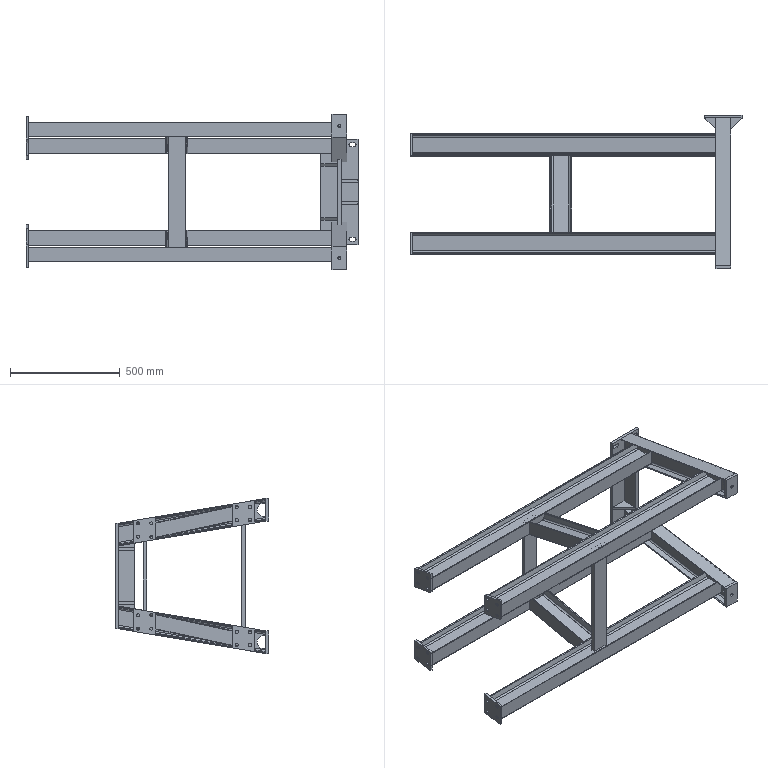Part | SolidWorks | 22 solids | 316 faces | box 1510 x 699 x 705.243 mm | volume 14014214 mm3 | plane 206 | cylinder 110 | commonest cylinder face diameters 5.6 x32 14 x32 14.8 x32 18 x8 13.835 x4 60 x2